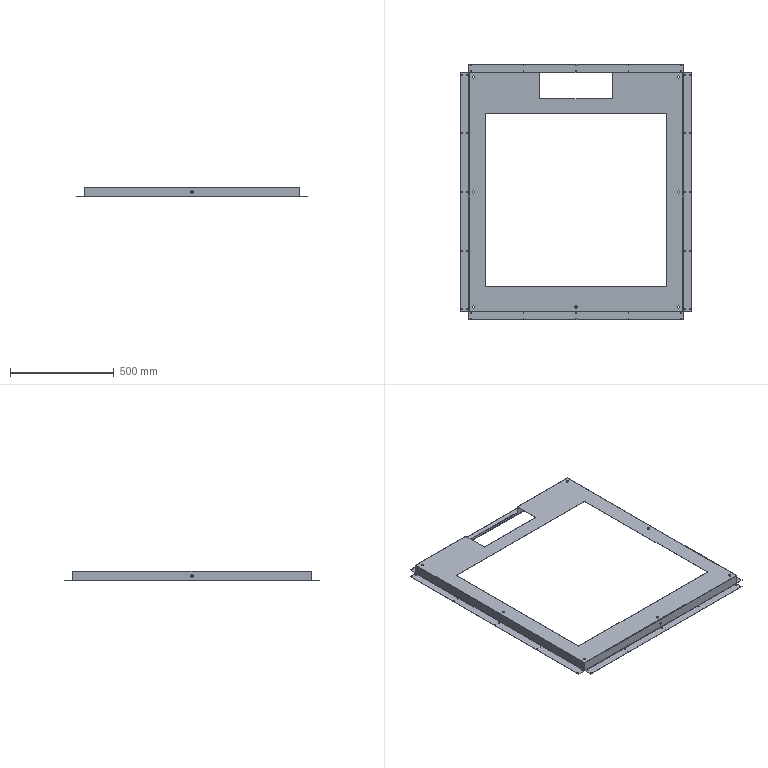Part | SolidWorks | features ICE 7, EdgeFlange 2, FlatPattern 1, SMBaseFlange 1, SheetMetal 1 | 1 solid | 184 faces | box 1113 x 1233 x 48 mm | volume 780188 mm3 | cylinder 118 | plane 58 | spline 8 | commonest cylinder face diameters 4.2 x80 11 x14 0.4 x9 2.4 x9 10 x6